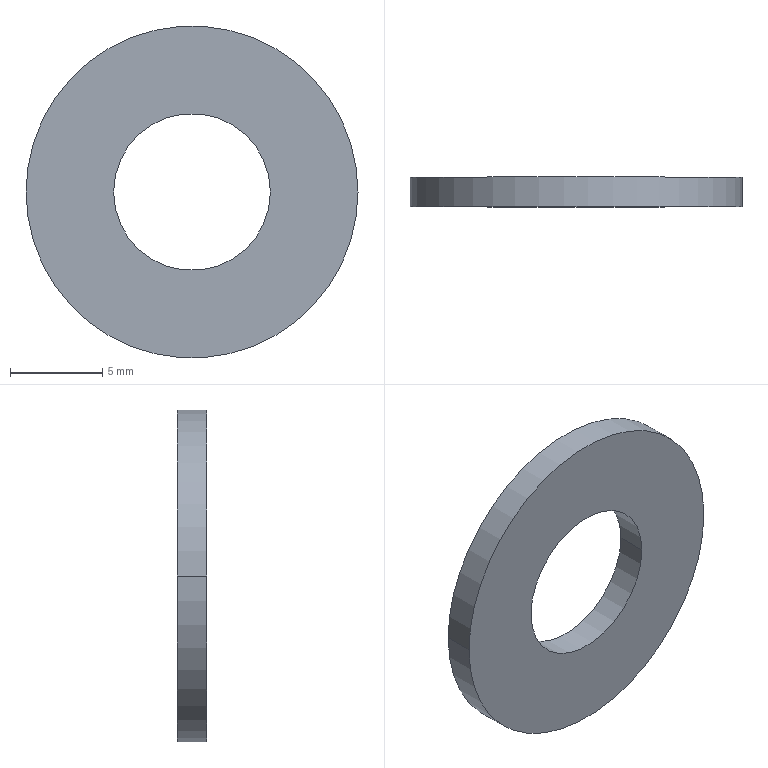Part | STEP file | ZZ21-M8 | 1 solid | 6 faces | box 18 x 1.6 x 18 mm | volume 316.358 mm3 | cylinder 4 | plane 2 | commonest cylinder face diameters 8.5 x2 18 x2
STEP:
#1=CARTESIAN_POINT('',(0.,0.,0.));
#2=DIRECTION('',(0.,0.,1.));
#3=DIRECTION('',(1.,0.,0.));
#4=AXIS2_PLACEMENT_3D('',#1,#2,#3);
#5=CARTESIAN_POINT('',(-9.,0.,0.));
#6=VERTEX_POINT('',#5);
#7=CARTESIAN_POINT('',(9.,0.,0.));
#8=VERTEX_POINT('',#7);
#9=CARTESIAN_POINT('',(0.,0.,0.));
#10=DIRECTION('',(0.,1.,0.));
#11=DIRECTION('',(-1.,0.,0.));
#12=AXIS2_PLACEMENT_3D('',#9,#10,#11);
#13=CIRCLE('',#12,9.);
#14=CARTESIAN_POINT('',(-19.092,0.,19.092));
#15=DIRECTION('',(0.,1.,0.));
#16=DIRECTION('',(1.,0.,0.));
#17=AXIS2_PLACEMENT_3D('',#14,#15,#16);
#18=PLANE('',#17);
#19=CARTESIAN_POINT('',(19.092,19.092));
#20=DIRECTION('',(-1.,0.));
#21=AXIS2_PLACEMENT_2D('',#19,#20);
#22=CIRCLE('',#21,9.);
#23=(GEOMETRIC_REPRESENTATION_CONTEXT(2)PARAMETRIC_REPRESENTATION_CONTEXT()REPRESENTATION_CONTEXT('',''));
#24=DEFINITIONAL_REPRESENTATION('',(#22),#23);
#25=PCURVE('',#18,#24);
#26=CARTESIAN_POINT('',(0.,0.8,0.));
#27=DIRECTION('',(0.,1.,0.));
#28=DIRECTION('',(1.,0.,0.));
#29=AXIS2_PLACEMENT_3D('',#26,#27,#28);
#30=CYLINDRICAL_SURFACE('',#29,9.);
#31=CARTESIAN_POINT('',(3.142,-0.8));
#32=DIRECTION('',(1.,0.));
#33=VECTOR('',#32,1.);
#34=LINE('',#31,#33);
#35=(GEOMETRIC_REPRESENTATION_CONTEXT(2)PARAMETRIC_REPRESENTATION_CONTEXT()REPRESENTATION_CONTEXT('',''));
#36=DEFINITIONAL_REPRESENTATION('',(#34),#35);
#37=PCURVE('',#30,#36);
#38=SURFACE_CURVE('',#13,(#25,#37),.PCURVE_S1.);
#39=EDGE_CURVE('',#6,#8,#38,.T.);
#40=ORIENTED_EDGE('',*,*,#39,.F.);
#41=CARTESIAN_POINT('',(0.,0.,0.));
#42=DIRECTION('',(0.,1.,0.));
#43=DIRECTION('',(1.,0.,0.));
#44=AXIS2_PLACEMENT_3D('',#41,#42,#43);
#45=CIRCLE('',#44,9.);
#46=CARTESIAN_POINT('',(19.092,19.092));
#47=DIRECTION('',(1.,0.));
#48=AXIS2_PLACEMENT_2D('',#46,#47);
#49=CIRCLE('',#48,9.);
#50=(GEOMETRIC_REPRESENTATION_CONTEXT(2)PARAMETRIC_REPRESENTATION_CONTEXT()REPRESENTATION_CONTEXT('',''));
#51=DEFINITIONAL_REPRESENTATION('',(#49),#50);
#52=PCURVE('',#18,#51);
#53=CARTESIAN_POINT('',(0.,0.8,0.));
#54=DIRECTION('',(0.,1.,0.));
#55=DIRECTION('',(1.,0.,0.));
#56=AXIS2_PLACEMENT_3D('',#53,#54,#55);
#57=CYLINDRICAL_SURFACE('',#56,9.);
#58=CARTESIAN_POINT('',(0.,-0.8));
#59=DIRECTION('',(1.,0.));
#60=VECTOR('',#59,1.);
#61=LINE('',#58,#60);
#62=(GEOMETRIC_REPRESENTATION_CONTEXT(2)PARAMETRIC_REPRESENTATION_CONTEXT()REPRESENTATION_CONTEXT('',''));
#63=DEFINITIONAL_REPRESENTATION('',(#61),#62);
#64=PCURVE('',#57,#63);
#65=SURFACE_CURVE('',#45,(#52,#64),.PCURVE_S1.);
#66=EDGE_CURVE('',#8,#6,#65,.T.);
#67=ORIENTED_EDGE('',*,*,#66,.F.);
#68=EDGE_LOOP('',(#40,#67));
#69=FACE_BOUND('',#68,.T.);
#70=CARTESIAN_POINT('',(-4.25,0.,0.));
#71=VERTEX_POINT('',#70);
#72=CARTESIAN_POINT('',(4.25,0.,0.));
#73=VERTEX_POINT('',#72);
#74=CARTESIAN_POINT('',(0.,0.,0.));
#75=DIRECTION('',(0.,-1.,0.));
#76=DIRECTION('',(-1.,0.,0.));
#77=AXIS2_PLACEMENT_3D('',#74,#75,#76);
#78=CIRCLE('',#77,4.25);
#79=CARTESIAN_POINT('',(14.842,19.092));
#80=CARTESIAN_POINT('',(14.842,26.453));
#81=CARTESIAN_POINT('',(21.217,22.772));
#82=CARTESIAN_POINT('',(27.592,19.092));
#83=CARTESIAN_POINT('',(21.217,15.411));
#84=CARTESIAN_POINT('',(14.842,11.731));
#85=CARTESIAN_POINT('',(14.842,19.092));
#86=(BOUNDED_CURVE()B_SPLINE_CURVE(2,(#79,#80,#81,#82,#83,#84,#85),.UNSPECIFIED.,.T.,.F.)B_SPLINE_CURVE_WITH_KNOTS((1,2,2,2,2,1),(-2.094,0.,2.094,4.189,6.283,8.378),.UNSPECIFIED.)CURVE()GEOMETRIC_REPRESENTATION_ITEM()RATIONAL_B_SPLINE_CURVE((1.,0.5,1.,0.5,1.,0.5,1.))REPRESENTATION_ITEM(''));
#87=(GEOMETRIC_REPRESENTATION_CONTEXT(2)PARAMETRIC_REPRESENTATION_CONTEXT()REPRESENTATION_CONTEXT('',''));
#88=DEFINITIONAL_REPRESENTATION('',(#86),#87);
#89=PCURVE('',#18,#88);
#90=CARTESIAN_POINT('',(0.,0.8,0.));
#91=DIRECTION('',(0.,1.,0.));
#92=DIRECTION('',(1.,0.,0.));
#93=AXIS2_PLACEMENT_3D('',#90,#91,#92);
#94=CYLINDRICAL_SURFACE('',#93,4.25);
#95=CARTESIAN_POINT('',(3.142,-0.8));
#96=DIRECTION('',(-1.,0.));
#97=VECTOR('',#96,1.);
#98=LINE('',#95,#97);
#99=(GEOMETRIC_REPRESENTATION_CONTEXT(2)PARAMETRIC_REPRESENTATION_CONTEXT()REPRESENTATION_CONTEXT('',''));
#100=DEFINITIONAL_REPRESENTATION('',(#98),#99);
#101=PCURVE('',#94,#100);
#102=SURFACE_CURVE('',#78,(#89,#101),.PCURVE_S1.);
#103=EDGE_CURVE('',#71,#73,#102,.T.);
#104=ORIENTED_EDGE('',*,*,#103,.F.);
#105=CARTESIAN_POINT('',(0.,0.,0.));
#106=DIRECTION('',(0.,-1.,0.));
#107=DIRECTION('',(1.,0.,0.));
#108=AXIS2_PLACEMENT_3D('',#105,#106,#107);
#109=CIRCLE('',#108,4.25);
#110=CARTESIAN_POINT('',(23.342,19.092));
#111=CARTESIAN_POINT('',(23.342,11.731));
#112=CARTESIAN_POINT('',(16.967,15.411));
#113=CARTESIAN_POINT('',(10.592,19.092));
#114=CARTESIAN_POINT('',(16.967,22.772));
#115=CARTESIAN_POINT('',(23.342,26.453));
#116=CARTESIAN_POINT('',(23.342,19.092));
#117=(BOUNDED_CURVE()B_SPLINE_CURVE(2,(#110,#111,#112,#113,#114,#115,#116),.UNSPECIFIED.,.T.,.F.)B_SPLINE_CURVE_WITH_KNOTS((1,2,2,2,2,1),(-2.094,0.,2.094,4.189,6.283,8.378),.UNSPECIFIED.)CURVE()GEOMETRIC_REPRESENTATION_ITEM()RATIONAL_B_SPLINE_CURVE((1.,0.5,1.,0.5,1.,0.5,1.))REPRESENTATION_ITEM(''));
#118=(GEOMETRIC_REPRESENTATION_CONTEXT(2)PARAMETRIC_REPRESENTATION_CONTEXT()REPRESENTATION_CONTEXT('',''));
#119=DEFINITIONAL_REPRESENTATION('',(#117),#118);
#120=PCURVE('',#18,#119);
#121=CARTESIAN_POINT('',(0.,0.8,0.));
#122=DIRECTION('',(0.,1.,0.));
#123=DIRECTION('',(1.,0.,0.));
#124=AXIS2_PLACEMENT_3D('',#121,#122,#123);
#125=CYLINDRICAL_SURFACE('',#124,4.25);
#126=CARTESIAN_POINT('',(6.283,-0.8));
#127=DIRECTION('',(-1.,0.));
#128=VECTOR('',#127,1.);
#129=LINE('',#126,#128);
#130=(GEOMETRIC_REPRESENTATION_CONTEXT(2)PARAMETRIC_REPRESENTATION_CONTEXT()REPRESENTATION_CONTEXT('',''));
#131=DEFINITIONAL_REPRESENTATION('',(#129),#130);
#132=PCURVE('',#125,#131);
#133=SURFACE_CURVE('',#109,(#120,#132),.PCURVE_S1.);
#134=EDGE_CURVE('',#73,#71,#133,.T.);
#135=ORIENTED_EDGE('',*,*,#134,.F.);
#136=EDGE_LOOP('',(#104,#135));
#137=FACE_BOUND('',#136,.T.);
#138=ADVANCED_FACE('',(#69,#137),#18,.F.);
#139=ORIENTED_EDGE('',*,*,#134,.F.);
#140=CARTESIAN_POINT('',(4.25,1.6,0.));
#141=VERTEX_POINT('',#140);
#142=CARTESIAN_POINT('',(4.25,0.,0.));
#143=DIRECTION('',(0.,1.,0.));
#144=VECTOR('',#143,1.);
#145=LINE('',#142,#144);
#146=CARTESIAN_POINT('',(6.283,-0.8));
#147=DIRECTION('',(0.,1.));
#148=VECTOR('',#147,1.);
#149=LINE('',#146,#148);
#150=(GEOMETRIC_REPRESENTATION_CONTEXT(2)PARAMETRIC_REPRESENTATION_CONTEXT()REPRESENTATION_CONTEXT('',''));
#151=DEFINITIONAL_REPRESENTATION('',(#149),#150);
#152=PCURVE('',#125,#151);
#153=CARTESIAN_POINT('',(0.,-0.8));
#154=DIRECTION('',(0.,1.));
#155=VECTOR('',#154,1.);
#156=LINE('',#153,#155);
#157=(GEOMETRIC_REPRESENTATION_CONTEXT(2)PARAMETRIC_REPRESENTATION_CONTEXT()REPRESENTATION_CONTEXT('',''));
#158=DEFINITIONAL_REPRESENTATION('',(#156),#157);
#159=PCURVE('',#94,#158);
#160=SURFACE_CURVE('',#145,(#152,#159),.PCURVE_S1.);
#161=EDGE_CURVE('',#73,#141,#160,.T.);
#162=ORIENTED_EDGE('',*,*,#161,.T.);
#163=CARTESIAN_POINT('',(-4.25,1.6,0.));
#164=VERTEX_POINT('',#163);
#165=CARTESIAN_POINT('',(0.,1.6,0.));
#166=DIRECTION('',(0.,-1.,0.));
#167=DIRECTION('',(1.,0.,0.));
#168=AXIS2_PLACEMENT_3D('',#165,#166,#167);
#169=CIRCLE('',#168,4.25);
#170=CARTESIAN_POINT('',(6.283,0.8));
#171=DIRECTION('',(-1.,0.));
#172=VECTOR('',#171,1.);
#173=LINE('',#170,#172);
#174=(GEOMETRIC_REPRESENTATION_CONTEXT(2)PARAMETRIC_REPRESENTATION_CONTEXT()REPRESENTATION_CONTEXT('',''));
#175=DEFINITIONAL_REPRESENTATION('',(#173),#174);
#176=PCURVE('',#125,#175);
#177=CARTESIAN_POINT('',(-19.092,1.6,19.092));
#178=DIRECTION('',(0.,1.,0.));
#179=DIRECTION('',(1.,0.,0.));
#180=AXIS2_PLACEMENT_3D('',#177,#178,#179);
#181=PLANE('',#180);
#182=CARTESIAN_POINT('',(23.342,19.092));
#183=CARTESIAN_POINT('',(23.342,11.731));
#184=CARTESIAN_POINT('',(16.967,15.411));
#185=CARTESIAN_POINT('',(10.592,19.092));
#186=CARTESIAN_POINT('',(16.967,22.772));
#187=CARTESIAN_POINT('',(23.342,26.453));
#188=CARTESIAN_POINT('',(23.342,19.092));
#189=(BOUNDED_CURVE()B_SPLINE_CURVE(2,(#182,#183,#184,#185,#186,#187,#188),.UNSPECIFIED.,.T.,.F.)B_SPLINE_CURVE_WITH_KNOTS((1,2,2,2,2,1),(-2.094,0.,2.094,4.189,6.283,8.378),.UNSPECIFIED.)CURVE()GEOMETRIC_REPRESENTATION_ITEM()RATIONAL_B_SPLINE_CURVE((1.,0.5,1.,0.5,1.,0.5,1.))REPRESENTATION_ITEM(''));
#190=(GEOMETRIC_REPRESENTATION_CONTEXT(2)PARAMETRIC_REPRESENTATION_CONTEXT()REPRESENTATION_CONTEXT('',''));
#191=DEFINITIONAL_REPRESENTATION('',(#189),#190);
#192=PCURVE('',#181,#191);
#193=SURFACE_CURVE('',#169,(#176,#192),.PCURVE_S1.);
#194=EDGE_CURVE('',#141,#164,#193,.T.);
#195=ORIENTED_EDGE('',*,*,#194,.T.);
#196=CARTESIAN_POINT('',(-4.25,0.,0.));
#197=DIRECTION('',(0.,1.,0.));
#198=VECTOR('',#197,1.);
#199=LINE('',#196,#198);
#200=CARTESIAN_POINT('',(3.142,-0.8));
#201=DIRECTION('',(0.,1.));
#202=VECTOR('',#201,1.);
#203=LINE('',#200,#202);
#204=(GEOMETRIC_REPRESENTATION_CONTEXT(2)PARAMETRIC_REPRESENTATION_CONTEXT()REPRESENTATION_CONTEXT('',''));
#205=DEFINITIONAL_REPRESENTATION('',(#203),#204);
#206=PCURVE('',#125,#205);
#207=CARTESIAN_POINT('',(3.142,-0.8));
#208=DIRECTION('',(0.,1.));
#209=VECTOR('',#208,1.);
#210=LINE('',#207,#209);
#211=(GEOMETRIC_REPRESENTATION_CONTEXT(2)PARAMETRIC_REPRESENTATION_CONTEXT()REPRESENTATION_CONTEXT('',''));
#212=DEFINITIONAL_REPRESENTATION('',(#210),#211);
#213=PCURVE('',#94,#212);
#214=SURFACE_CURVE('',#199,(#206,#213),.PCURVE_S1.);
#215=EDGE_CURVE('',#71,#164,#214,.T.);
#216=ORIENTED_EDGE('',*,*,#215,.F.);
#217=EDGE_LOOP('',(#139,#162,#195,#216));
#218=FACE_BOUND('',#217,.F.);
#219=ADVANCED_FACE('',(#218),#125,.F.);
#220=ORIENTED_EDGE('',*,*,#103,.F.);
#221=ORIENTED_EDGE('',*,*,#215,.T.);
#222=CARTESIAN_POINT('',(0.,1.6,0.));
#223=DIRECTION('',(0.,-1.,0.));
#224=DIRECTION('',(-1.,0.,0.));
#225=AXIS2_PLACEMENT_3D('',#222,#223,#224);
#226=CIRCLE('',#225,4.25);
#227=CARTESIAN_POINT('',(3.142,0.8));
#228=DIRECTION('',(-1.,0.));
#229=VECTOR('',#228,1.);
#230=LINE('',#227,#229);
#231=(GEOMETRIC_REPRESENTATION_CONTEXT(2)PARAMETRIC_REPRESENTATION_CONTEXT()REPRESENTATION_CONTEXT('',''));
#232=DEFINITIONAL_REPRESENTATION('',(#230),#231);
#233=PCURVE('',#94,#232);
#234=CARTESIAN_POINT('',(14.842,19.092));
#235=CARTESIAN_POINT('',(14.842,26.453));
#236=CARTESIAN_POINT('',(21.217,22.772));
#237=CARTESIAN_POINT('',(27.592,19.092));
#238=CARTESIAN_POINT('',(21.217,15.411));
#239=CARTESIAN_POINT('',(14.842,11.731));
#240=CARTESIAN_POINT('',(14.842,19.092));
#241=(BOUNDED_CURVE()B_SPLINE_CURVE(2,(#234,#235,#236,#237,#238,#239,#240),.UNSPECIFIED.,.T.,.F.)B_SPLINE_CURVE_WITH_KNOTS((1,2,2,2,2,1),(-2.094,0.,2.094,4.189,6.283,8.378),.UNSPECIFIED.)CURVE()GEOMETRIC_REPRESENTATION_ITEM()RATIONAL_B_SPLINE_CURVE((1.,0.5,1.,0.5,1.,0.5,1.))REPRESENTATION_ITEM(''));
#242=(GEOMETRIC_REPRESENTATION_CONTEXT(2)PARAMETRIC_REPRESENTATION_CONTEXT()REPRESENTATION_CONTEXT('',''));
#243=DEFINITIONAL_REPRESENTATION('',(#241),#242);
#244=PCURVE('',#181,#243);
#245=SURFACE_CURVE('',#226,(#233,#244),.PCURVE_S1.);
#246=EDGE_CURVE('',#164,#141,#245,.T.);
#247=ORIENTED_EDGE('',*,*,#246,.T.);
#248=ORIENTED_EDGE('',*,*,#161,.F.);
#249=EDGE_LOOP('',(#220,#221,#247,#248));
#250=FACE_BOUND('',#249,.F.);
#251=ADVANCED_FACE('',(#250),#94,.F.);
#252=CARTESIAN_POINT('',(-9.,1.6,0.));
#253=VERTEX_POINT('',#252);
#254=CARTESIAN_POINT('',(9.,1.6,0.));
#255=VERTEX_POINT('',#254);
#256=CARTESIAN_POINT('',(0.,1.6,0.));
#257=DIRECTION('',(0.,1.,0.));
#258=DIRECTION('',(-1.,0.,0.));
#259=AXIS2_PLACEMENT_3D('',#256,#257,#258);
#260=CIRCLE('',#259,9.);
#261=CARTESIAN_POINT('',(19.092,19.092));
#262=DIRECTION('',(-1.,0.));
#263=AXIS2_PLACEMENT_2D('',#261,#262);
#264=CIRCLE('',#263,9.);
#265=(GEOMETRIC_REPRESENTATION_CONTEXT(2)PARAMETRIC_REPRESENTATION_CONTEXT()REPRESENTATION_CONTEXT('',''));
#266=DEFINITIONAL_REPRESENTATION('',(#264),#265);
#267=PCURVE('',#181,#266);
#268=CARTESIAN_POINT('',(3.142,0.8));
#269=DIRECTION('',(1.,0.));
#270=VECTOR('',#269,1.);
#271=LINE('',#268,#270);
#272=(GEOMETRIC_REPRESENTATION_CONTEXT(2)PARAMETRIC_REPRESENTATION_CONTEXT()REPRESENTATION_CONTEXT('',''));
#273=DEFINITIONAL_REPRESENTATION('',(#271),#272);
#274=PCURVE('',#30,#273);
#275=SURFACE_CURVE('',#260,(#267,#274),.PCURVE_S1.);
#276=EDGE_CURVE('',#253,#255,#275,.T.);
#277=ORIENTED_EDGE('',*,*,#276,.T.);
#278=CARTESIAN_POINT('',(0.,1.6,0.));
#279=DIRECTION('',(0.,1.,0.));
#280=DIRECTION('',(1.,0.,0.));
#281=AXIS2_PLACEMENT_3D('',#278,#279,#280);
#282=CIRCLE('',#281,9.);
#283=CARTESIAN_POINT('',(19.092,19.092));
#284=DIRECTION('',(1.,0.));
#285=AXIS2_PLACEMENT_2D('',#283,#284);
#286=CIRCLE('',#285,9.);
#287=(GEOMETRIC_REPRESENTATION_CONTEXT(2)PARAMETRIC_REPRESENTATION_CONTEXT()REPRESENTATION_CONTEXT('',''));
#288=DEFINITIONAL_REPRESENTATION('',(#286),#287);
#289=PCURVE('',#181,#288);
#290=CARTESIAN_POINT('',(0.,0.8));
#291=DIRECTION('',(1.,0.));
#292=VECTOR('',#291,1.);
#293=LINE('',#290,#292);
#294=(GEOMETRIC_REPRESENTATION_CONTEXT(2)PARAMETRIC_REPRESENTATION_CONTEXT()REPRESENTATION_CONTEXT('',''));
#295=DEFINITIONAL_REPRESENTATION('',(#293),#294);
#296=PCURVE('',#57,#295);
#297=SURFACE_CURVE('',#282,(#289,#296),.PCURVE_S1.);
#298=EDGE_CURVE('',#255,#253,#297,.T.);
#299=ORIENTED_EDGE('',*,*,#298,.T.);
#300=EDGE_LOOP('',(#277,#299));
#301=FACE_BOUND('',#300,.T.);
#302=ORIENTED_EDGE('',*,*,#246,.T.);
#303=ORIENTED_EDGE('',*,*,#194,.T.);
#304=EDGE_LOOP('',(#302,#303));
#305=FACE_BOUND('',#304,.T.);
#306=ADVANCED_FACE('',(#301,#305),#181,.T.);
#307=CARTESIAN_POINT('',(-9.,0.,0.));
#308=DIRECTION('',(0.,1.,0.));
#309=VECTOR('',#308,1.);
#310=LINE('',#307,#309);
#311=CARTESIAN_POINT('',(3.142,-0.8));
#312=DIRECTION('',(0.,1.));
#313=VECTOR('',#312,1.);
#314=LINE('',#311,#313);
#315=(GEOMETRIC_REPRESENTATION_CONTEXT(2)PARAMETRIC_REPRESENTATION_CONTEXT()REPRESENTATION_CONTEXT('',''));
#316=DEFINITIONAL_REPRESENTATION('',(#314),#315);
#317=PCURVE('',#57,#316);
#318=CARTESIAN_POINT('',(3.142,-0.8));
#319=DIRECTION('',(0.,1.));
#320=VECTOR('',#319,1.);
#321=LINE('',#318,#320);
#322=(GEOMETRIC_REPRESENTATION_CONTEXT(2)PARAMETRIC_REPRESENTATION_CONTEXT()REPRESENTATION_CONTEXT('',''));
#323=DEFINITIONAL_REPRESENTATION('',(#321),#322);
#324=PCURVE('',#30,#323);
#325=SURFACE_CURVE('',#310,(#317,#324),.PCURVE_S1.);
#326=EDGE_CURVE('',#6,#253,#325,.T.);
#327=ORIENTED_EDGE('',*,*,#326,.T.);
#328=ORIENTED_EDGE('',*,*,#298,.F.);
#329=CARTESIAN_POINT('',(9.,0.,0.));
#330=DIRECTION('',(0.,1.,0.));
#331=VECTOR('',#330,1.);
#332=LINE('',#329,#331);
#333=CARTESIAN_POINT('',(0.,-0.8));
#334=DIRECTION('',(0.,1.));
#335=VECTOR('',#334,1.);
#336=LINE('',#333,#335);
#337=(GEOMETRIC_REPRESENTATION_CONTEXT(2)PARAMETRIC_REPRESENTATION_CONTEXT()REPRESENTATION_CONTEXT('',''));
#338=DEFINITIONAL_REPRESENTATION('',(#336),#337);
#339=PCURVE('',#57,#338);
#340=CARTESIAN_POINT('',(6.283,-0.8));
#341=DIRECTION('',(0.,1.));
#342=VECTOR('',#341,1.);
#343=LINE('',#340,#342);
#344=(GEOMETRIC_REPRESENTATION_CONTEXT(2)PARAMETRIC_REPRESENTATION_CONTEXT()REPRESENTATION_CONTEXT('',''));
#345=DEFINITIONAL_REPRESENTATION('',(#343),#344);
#346=PCURVE('',#30,#345);
#347=SURFACE_CURVE('',#332,(#339,#346),.PCURVE_S1.);
#348=EDGE_CURVE('',#8,#255,#347,.T.);
#349=ORIENTED_EDGE('',*,*,#348,.F.);
#350=ORIENTED_EDGE('',*,*,#66,.T.);
#351=EDGE_LOOP('',(#327,#328,#349,#350));
#352=FACE_BOUND('',#351,.T.);
#353=ADVANCED_FACE('',(#352),#57,.T.);
#354=ORIENTED_EDGE('',*,*,#348,.T.);
#355=ORIENTED_EDGE('',*,*,#276,.F.);
#356=ORIENTED_EDGE('',*,*,#326,.F.);
#357=ORIENTED_EDGE('',*,*,#39,.T.);
#358=EDGE_LOOP('',(#354,#355,#356,#357));
#359=FACE_BOUND('',#358,.T.);
#360=ADVANCED_FACE('',(#359),#30,.T.);
#361=CLOSED_SHELL('',(#138,#219,#251,#306,#353,#360));
#362=MANIFOLD_SOLID_BREP('',#361);
#363=(LENGTH_UNIT()NAMED_UNIT(*)SI_UNIT(.MILLI.,.METRE.));
#364=UNCERTAINTY_MEASURE_WITH_UNIT(LENGTH_MEASURE(0.0000001),#363,'','');
#365=(NAMED_UNIT(*)PLANE_ANGLE_UNIT()SI_UNIT($,.RADIAN.));
#366=(NAMED_UNIT(*)SI_UNIT($,.STERADIAN.)SOLID_ANGLE_UNIT());
#367=(GEOMETRIC_REPRESENTATION_CONTEXT(3)GLOBAL_UNCERTAINTY_ASSIGNED_CONTEXT((#364))GLOBAL_UNIT_ASSIGNED_CONTEXT((#363,#365,#366))REPRESENTATION_CONTEXT('',''));
#368=ADVANCED_BREP_SHAPE_REPRESENTATION('',(#4,#362),#367);